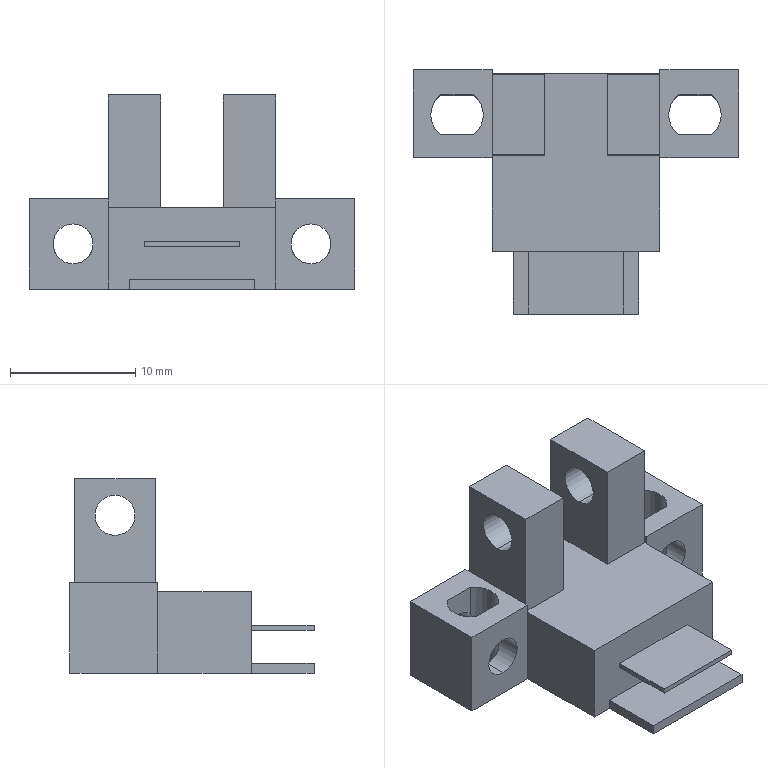Part | STEP file | 0244_011_FPML54 | 1 solid | 63 faces | box 26 x 19.5 x 15.5 mm | volume 2111 mm3 | plane 45 | cylinder 18 | commonest cylinder face diameters 3.2 x12 4 x6